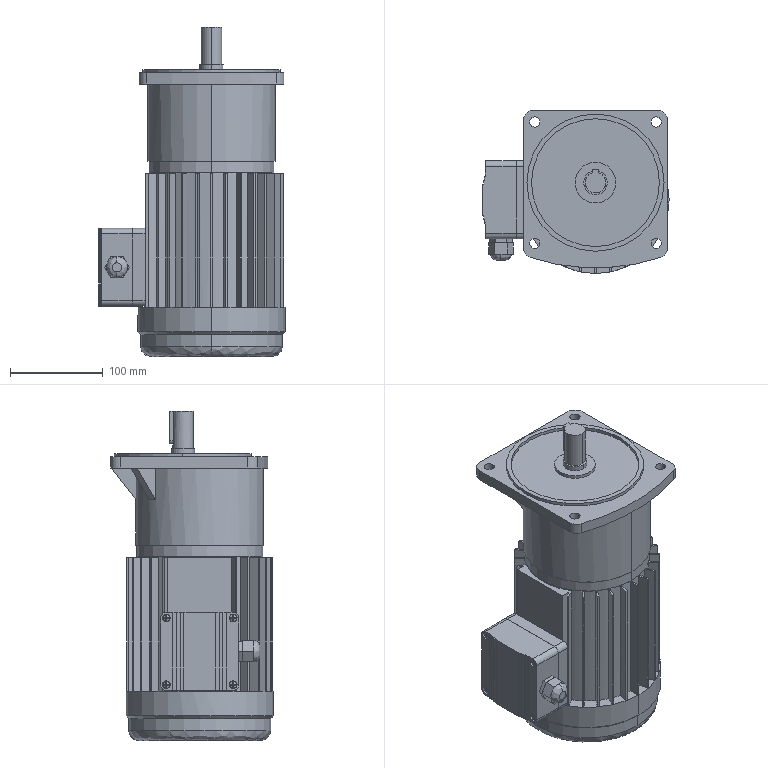Part | SolidWorks | features BaseBody 2 | 2 solids | 558 faces | box 201.05 x 175.7 x 355 mm | volume 5359674 mm3 | plane 465 | cylinder 75 | spline 16 | cone 2 | commonest cylinder face diameters 22 x14 8 x8 8.5 x8 11 x8 12 x8 10 x4